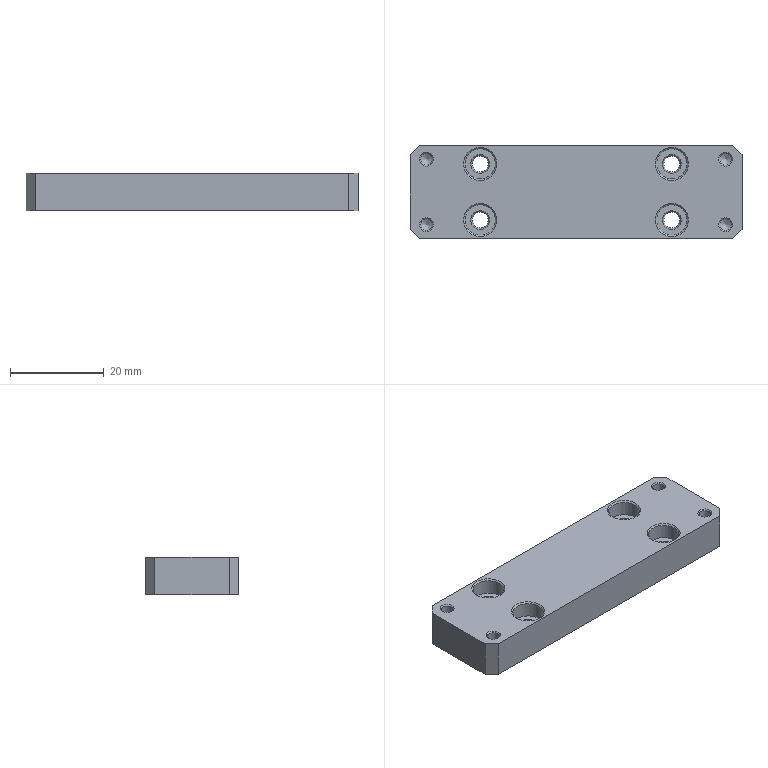Part | NX | features CBORE_HOLE 4, DATUM_CSYS 4, LINKED_CURVE 4, SIMPLE HOLE 4, SYMBOLIC_THREAD 4, SKETCH 3, HOLE PACKAGE 2, CHAMFER 1, EXTRUDE 1, LINKED_FACE 1 | 1 solid | 46 faces | box 71 x 20 x 8 mm | volume 10535 mm3 | cone 20 | plane 14 | cylinder 12 | commonest cylinder face diameters 2.5 x4 3.4 x4 6.5 x4
STEP:
#1=CARTESIAN_POINT('',(-608.186,976.556,396.282));
#2=VERTEX_POINT('',#1);
#3=CARTESIAN_POINT('',(-608.186,992.556,396.282));
#4=VERTEX_POINT('',#3);
#5=CARTESIAN_POINT('',(-608.186,974.556,396.282));
#6=DIRECTION('',(0.,1.,0.));
#7=VECTOR('',#6,1000.);
#8=LINE('',#5,#7);
#9=EDGE_CURVE('',#2,#4,#8,.T.);
#10=ORIENTED_EDGE('',*,*,#9,.T.);
#11=CARTESIAN_POINT('',(-608.186,992.556,388.282));
#12=VERTEX_POINT('',#11);
#13=CARTESIAN_POINT('',(-608.186,992.556,388.282));
#14=DIRECTION('',(0.,0.,-1.));
#15=VECTOR('',#14,1000.);
#16=LINE('',#13,#15);
#17=EDGE_CURVE('',#4,#12,#16,.T.);
#18=ORIENTED_EDGE('',*,*,#17,.T.);
#19=CARTESIAN_POINT('',(-608.186,976.556,388.282));
#20=VERTEX_POINT('',#19);
#21=CARTESIAN_POINT('',(-608.186,974.556,388.282));
#22=DIRECTION('',(0.,1.,0.));
#23=VECTOR('',#22,1000.);
#24=LINE('',#21,#23);
#25=EDGE_CURVE('',#20,#12,#24,.T.);
#26=ORIENTED_EDGE('',*,*,#25,.F.);
#27=CARTESIAN_POINT('',(-608.186,976.556,388.282));
#28=DIRECTION('',(0.,0.,1.));
#29=VECTOR('',#28,1000.);
#30=LINE('',#27,#29);
#31=EDGE_CURVE('',#20,#2,#30,.T.);
#32=ORIENTED_EDGE('',*,*,#31,.T.);
#33=EDGE_LOOP('',(#10,#18,#26,#32));
#34=FACE_BOUND('',#33,.T.);
#35=CARTESIAN_POINT('',(-608.186,974.556,388.282));
#36=DIRECTION('',(1.,0.,0.));
#37=DIRECTION('',(0.,0.,-1.));
#38=AXIS2_PLACEMENT_3D('',#35,#36,#37);
#39=PLANE('',#38);
#40=ADVANCED_FACE('',(#34),#39,.F.);
#41=CARTESIAN_POINT('',(-606.186,994.556,396.282));
#42=VERTEX_POINT('',#41);
#43=CARTESIAN_POINT('',(-539.186,994.556,396.282));
#44=VERTEX_POINT('',#43);
#45=CARTESIAN_POINT('',(-608.186,994.556,396.282));
#46=DIRECTION('',(1.,0.,0.));
#47=VECTOR('',#46,1000.);
#48=LINE('',#45,#47);
#49=EDGE_CURVE('',#42,#44,#48,.T.);
#50=ORIENTED_EDGE('',*,*,#49,.T.);
#51=CARTESIAN_POINT('',(-539.186,994.556,388.282));
#52=VERTEX_POINT('',#51);
#53=CARTESIAN_POINT('',(-539.186,994.556,388.282));
#54=DIRECTION('',(0.,0.,-1.));
#55=VECTOR('',#54,1000.);
#56=LINE('',#53,#55);
#57=EDGE_CURVE('',#44,#52,#56,.T.);
#58=ORIENTED_EDGE('',*,*,#57,.T.);
#59=CARTESIAN_POINT('',(-606.186,994.556,388.282));
#60=VERTEX_POINT('',#59);
#61=CARTESIAN_POINT('',(-608.186,994.556,388.282));
#62=DIRECTION('',(1.,0.,0.));
#63=VECTOR('',#62,1000.);
#64=LINE('',#61,#63);
#65=EDGE_CURVE('',#60,#52,#64,.T.);
#66=ORIENTED_EDGE('',*,*,#65,.F.);
#67=CARTESIAN_POINT('',(-606.186,994.556,388.282));
#68=DIRECTION('',(0.,0.,1.));
#69=VECTOR('',#68,1000.);
#70=LINE('',#67,#69);
#71=EDGE_CURVE('',#60,#42,#70,.T.);
#72=ORIENTED_EDGE('',*,*,#71,.T.);
#73=EDGE_LOOP('',(#50,#58,#66,#72));
#74=FACE_BOUND('',#73,.T.);
#75=CARTESIAN_POINT('',(-608.186,994.556,388.282));
#76=DIRECTION('',(0.,-1.,0.));
#77=DIRECTION('',(0.,0.,-1.));
#78=AXIS2_PLACEMENT_3D('',#75,#76,#77);
#79=PLANE('',#78);
#80=ADVANCED_FACE('',(#74),#79,.F.);
#81=CARTESIAN_POINT('',(-537.186,992.556,388.282));
#82=VERTEX_POINT('',#81);
#83=CARTESIAN_POINT('',(-537.186,976.556,388.282));
#84=VERTEX_POINT('',#83);
#85=CARTESIAN_POINT('',(-537.186,994.556,388.282));
#86=DIRECTION('',(0.,-1.,0.));
#87=VECTOR('',#86,1000.);
#88=LINE('',#85,#87);
#89=EDGE_CURVE('',#82,#84,#88,.T.);
#90=ORIENTED_EDGE('',*,*,#89,.F.);
#91=CARTESIAN_POINT('',(-537.186,992.556,396.282));
#92=VERTEX_POINT('',#91);
#93=CARTESIAN_POINT('',(-537.186,992.556,388.282));
#94=DIRECTION('',(0.,0.,1.));
#95=VECTOR('',#94,1000.);
#96=LINE('',#93,#95);
#97=EDGE_CURVE('',#82,#92,#96,.T.);
#98=ORIENTED_EDGE('',*,*,#97,.T.);
#99=CARTESIAN_POINT('',(-537.186,976.556,396.282));
#100=VERTEX_POINT('',#99);
#101=CARTESIAN_POINT('',(-537.186,994.556,396.282));
#102=DIRECTION('',(0.,-1.,0.));
#103=VECTOR('',#102,1000.);
#104=LINE('',#101,#103);
#105=EDGE_CURVE('',#92,#100,#104,.T.);
#106=ORIENTED_EDGE('',*,*,#105,.T.);
#107=CARTESIAN_POINT('',(-537.186,976.556,388.282));
#108=DIRECTION('',(0.,0.,-1.));
#109=VECTOR('',#108,1000.);
#110=LINE('',#107,#109);
#111=EDGE_CURVE('',#100,#84,#110,.T.);
#112=ORIENTED_EDGE('',*,*,#111,.T.);
#113=EDGE_LOOP('',(#90,#98,#106,#112));
#114=FACE_BOUND('',#113,.T.);
#115=CARTESIAN_POINT('',(-537.186,994.556,388.282));
#116=DIRECTION('',(-1.,0.,0.));
#117=DIRECTION('',(0.,0.,1.));
#118=AXIS2_PLACEMENT_3D('',#115,#116,#117);
#119=PLANE('',#118);
#120=ADVANCED_FACE('',(#114),#119,.F.);
#121=CARTESIAN_POINT('',(-539.186,974.556,388.282));
#122=VERTEX_POINT('',#121);
#123=CARTESIAN_POINT('',(-606.186,974.556,388.282));
#124=VERTEX_POINT('',#123);
#125=CARTESIAN_POINT('',(-537.186,974.556,388.282));
#126=DIRECTION('',(-1.,0.,0.));
#127=VECTOR('',#126,1000.);
#128=LINE('',#125,#127);
#129=EDGE_CURVE('',#122,#124,#128,.T.);
#130=ORIENTED_EDGE('',*,*,#129,.F.);
#131=CARTESIAN_POINT('',(-539.186,974.556,396.282));
#132=VERTEX_POINT('',#131);
#133=CARTESIAN_POINT('',(-539.186,974.556,388.282));
#134=DIRECTION('',(0.,0.,1.));
#135=VECTOR('',#134,1000.);
#136=LINE('',#133,#135);
#137=EDGE_CURVE('',#122,#132,#136,.T.);
#138=ORIENTED_EDGE('',*,*,#137,.T.);
#139=CARTESIAN_POINT('',(-606.186,974.556,396.282));
#140=VERTEX_POINT('',#139);
#141=CARTESIAN_POINT('',(-537.186,974.556,396.282));
#142=DIRECTION('',(-1.,0.,0.));
#143=VECTOR('',#142,1000.);
#144=LINE('',#141,#143);
#145=EDGE_CURVE('',#132,#140,#144,.T.);
#146=ORIENTED_EDGE('',*,*,#145,.T.);
#147=CARTESIAN_POINT('',(-606.186,974.556,388.282));
#148=DIRECTION('',(0.,0.,-1.));
#149=VECTOR('',#148,1000.);
#150=LINE('',#147,#149);
#151=EDGE_CURVE('',#140,#124,#150,.T.);
#152=ORIENTED_EDGE('',*,*,#151,.T.);
#153=EDGE_LOOP('',(#130,#138,#146,#152));
#154=FACE_BOUND('',#153,.T.);
#155=CARTESIAN_POINT('',(-537.186,974.556,388.282));
#156=DIRECTION('',(0.,1.,0.));
#157=DIRECTION('',(0.,0.,1.));
#158=AXIS2_PLACEMENT_3D('',#155,#156,#157);
#159=PLANE('',#158);
#160=ADVANCED_FACE('',(#154),#159,.F.);
#161=CARTESIAN_POINT('',(-554.186,978.556,388.282));
#162=VERTEX_POINT('',#161);
#163=CARTESIAN_POINT('',(-552.186,978.556,388.282));
#164=DIRECTION('',(0.,0.,-1.));
#165=DIRECTION('',(-1.,0.,0.));
#166=AXIS2_PLACEMENT_3D('',#163,#164,#165);
#167=CIRCLE('',#166,2.);
#168=EDGE_CURVE('',#162,#162,#167,.F.);
#169=ORIENTED_EDGE('',*,*,#168,.T.);
#170=EDGE_LOOP('',(#169));
#171=FACE_BOUND('',#170,.T.);
#172=CARTESIAN_POINT('',(-554.186,990.556,388.282));
#173=VERTEX_POINT('',#172);
#174=CARTESIAN_POINT('',(-552.186,990.556,388.282));
#175=DIRECTION('',(0.,0.,-1.));
#176=DIRECTION('',(-1.,0.,0.));
#177=AXIS2_PLACEMENT_3D('',#174,#175,#176);
#178=CIRCLE('',#177,2.);
#179=EDGE_CURVE('',#173,#173,#178,.F.);
#180=ORIENTED_EDGE('',*,*,#179,.T.);
#181=EDGE_LOOP('',(#180));
#182=FACE_BOUND('',#181,.T.);
#183=CARTESIAN_POINT('',(-595.186,978.556,388.282));
#184=VERTEX_POINT('',#183);
#185=CARTESIAN_POINT('',(-593.186,978.556,388.282));
#186=DIRECTION('',(0.,0.,-1.));
#187=DIRECTION('',(-1.,0.,0.));
#188=AXIS2_PLACEMENT_3D('',#185,#186,#187);
#189=CIRCLE('',#188,2.);
#190=EDGE_CURVE('',#184,#184,#189,.F.);
#191=ORIENTED_EDGE('',*,*,#190,.T.);
#192=EDGE_LOOP('',(#191));
#193=FACE_BOUND('',#192,.T.);
#194=CARTESIAN_POINT('',(-595.186,990.556,388.282));
#195=VERTEX_POINT('',#194);
#196=CARTESIAN_POINT('',(-593.186,990.556,388.282));
#197=DIRECTION('',(0.,0.,-1.));
#198=DIRECTION('',(-1.,0.,0.));
#199=AXIS2_PLACEMENT_3D('',#196,#197,#198);
#200=CIRCLE('',#199,2.);
#201=EDGE_CURVE('',#195,#195,#200,.F.);
#202=ORIENTED_EDGE('',*,*,#201,.T.);
#203=EDGE_LOOP('',(#202));
#204=FACE_BOUND('',#203,.T.);
#205=ORIENTED_EDGE('',*,*,#65,.T.);
#206=CARTESIAN_POINT('',(227.685,227.685,388.282));
#207=DIRECTION('',(-0.7071,0.7071,0.));
#208=VECTOR('',#207,1000.);
#209=LINE('',#206,#208);
#210=EDGE_CURVE('',#52,#82,#209,.F.);
#211=ORIENTED_EDGE('',*,*,#210,.T.);
#212=ORIENTED_EDGE('',*,*,#89,.T.);
#213=CARTESIAN_POINT('',(-756.871,756.871,388.282));
#214=DIRECTION('',(0.7071,0.7071,0.));
#215=VECTOR('',#214,1000.);
#216=LINE('',#213,#215);
#217=EDGE_CURVE('',#84,#122,#216,.F.);
#218=ORIENTED_EDGE('',*,*,#217,.T.);
#219=ORIENTED_EDGE('',*,*,#129,.T.);
#220=CARTESIAN_POINT('',(184.185,184.185,388.282));
#221=DIRECTION('',(0.7071,-0.7071,0.));
#222=VECTOR('',#221,1000.);
#223=LINE('',#220,#222);
#224=EDGE_CURVE('',#124,#20,#223,.F.);
#225=ORIENTED_EDGE('',*,*,#224,.T.);
#226=ORIENTED_EDGE('',*,*,#25,.T.);
#227=CARTESIAN_POINT('',(-800.371,800.371,388.282));
#228=DIRECTION('',(-0.7071,-0.7071,0.));
#229=VECTOR('',#228,1000.);
#230=LINE('',#227,#229);
#231=EDGE_CURVE('',#12,#60,#230,.F.);
#232=ORIENTED_EDGE('',*,*,#231,.T.);
#233=EDGE_LOOP('',(#205,#211,#212,#218,#219,#225,#226,#232));
#234=FACE_BOUND('',#233,.T.);
#235=CARTESIAN_POINT('',(0.,0.,388.282));
#236=DIRECTION('',(0.,0.,-1.));
#237=DIRECTION('',(-1.,0.,0.));
#238=AXIS2_PLACEMENT_3D('',#235,#236,#237);
#239=PLANE('',#238);
#240=ADVANCED_FACE('',(#171,#182,#193,#204,#234),#239,.T.);
#241=CARTESIAN_POINT('',(-555.736,978.556,396.282));
#242=VERTEX_POINT('',#241);
#243=CARTESIAN_POINT('',(-552.186,978.556,396.282));
#244=DIRECTION('',(0.,0.,-1.));
#245=DIRECTION('',(-1.,0.,0.));
#246=AXIS2_PLACEMENT_3D('',#243,#244,#245);
#247=CIRCLE('',#246,3.55);
#248=EDGE_CURVE('',#242,#242,#247,.T.);
#249=ORIENTED_EDGE('',*,*,#248,.T.);
#250=EDGE_LOOP('',(#249));
#251=FACE_BOUND('',#250,.T.);
#252=CARTESIAN_POINT('',(-555.736,990.556,396.282));
#253=VERTEX_POINT('',#252);
#254=CARTESIAN_POINT('',(-552.186,990.556,396.282));
#255=DIRECTION('',(0.,0.,-1.));
#256=DIRECTION('',(-1.,0.,0.));
#257=AXIS2_PLACEMENT_3D('',#254,#255,#256);
#258=CIRCLE('',#257,3.55);
#259=EDGE_CURVE('',#253,#253,#258,.T.);
#260=ORIENTED_EDGE('',*,*,#259,.T.);
#261=EDGE_LOOP('',(#260));
#262=FACE_BOUND('',#261,.T.);
#263=CARTESIAN_POINT('',(-596.736,978.556,396.282));
#264=VERTEX_POINT('',#263);
#265=CARTESIAN_POINT('',(-593.186,978.556,396.282));
#266=DIRECTION('',(0.,0.,-1.));
#267=DIRECTION('',(-1.,0.,0.));
#268=AXIS2_PLACEMENT_3D('',#265,#266,#267);
#269=CIRCLE('',#268,3.55);
#270=EDGE_CURVE('',#264,#264,#269,.T.);
#271=ORIENTED_EDGE('',*,*,#270,.T.);
#272=EDGE_LOOP('',(#271));
#273=FACE_BOUND('',#272,.T.);
#274=CARTESIAN_POINT('',(-596.736,990.556,396.282));
#275=VERTEX_POINT('',#274);
#276=CARTESIAN_POINT('',(-593.186,990.556,396.282));
#277=DIRECTION('',(0.,0.,-1.));
#278=DIRECTION('',(-1.,0.,0.));
#279=AXIS2_PLACEMENT_3D('',#276,#277,#278);
#280=CIRCLE('',#279,3.55);
#281=EDGE_CURVE('',#275,#275,#280,.T.);
#282=ORIENTED_EDGE('',*,*,#281,.T.);
#283=EDGE_LOOP('',(#282));
#284=FACE_BOUND('',#283,.T.);
#285=CARTESIAN_POINT('',(-542.186,977.556,396.282));
#286=VERTEX_POINT('',#285);
#287=CARTESIAN_POINT('',(-540.686,977.556,396.282));
#288=DIRECTION('',(0.,0.,-1.));
#289=DIRECTION('',(-1.,0.,0.));
#290=AXIS2_PLACEMENT_3D('',#287,#288,#289);
#291=CIRCLE('',#290,1.5);
#292=EDGE_CURVE('',#286,#286,#291,.T.);
#293=ORIENTED_EDGE('',*,*,#292,.T.);
#294=EDGE_LOOP('',(#293));
#295=FACE_BOUND('',#294,.T.);
#296=CARTESIAN_POINT('',(-542.186,991.556,396.282));
#297=VERTEX_POINT('',#296);
#298=CARTESIAN_POINT('',(-540.686,991.556,396.282));
#299=DIRECTION('',(0.,0.,-1.));
#300=DIRECTION('',(-1.,0.,0.));
#301=AXIS2_PLACEMENT_3D('',#298,#299,#300);
#302=CIRCLE('',#301,1.5);
#303=EDGE_CURVE('',#297,#297,#302,.T.);
#304=ORIENTED_EDGE('',*,*,#303,.T.);
#305=EDGE_LOOP('',(#304));
#306=FACE_BOUND('',#305,.T.);
#307=CARTESIAN_POINT('',(-606.186,977.561,396.282));
#308=VERTEX_POINT('',#307);
#309=CARTESIAN_POINT('',(-604.686,977.561,396.282));
#310=DIRECTION('',(0.,0.,-1.));
#311=DIRECTION('',(-1.,0.,0.));
#312=AXIS2_PLACEMENT_3D('',#309,#310,#311);
#313=CIRCLE('',#312,1.5);
#314=EDGE_CURVE('',#308,#308,#313,.T.);
#315=ORIENTED_EDGE('',*,*,#314,.T.);
#316=EDGE_LOOP('',(#315));
#317=FACE_BOUND('',#316,.T.);
#318=CARTESIAN_POINT('',(-606.186,991.561,396.282));
#319=VERTEX_POINT('',#318);
#320=CARTESIAN_POINT('',(-604.686,991.561,396.282));
#321=DIRECTION('',(0.,0.,-1.));
#322=DIRECTION('',(-1.,0.,0.));
#323=AXIS2_PLACEMENT_3D('',#320,#321,#322);
#324=CIRCLE('',#323,1.5);
#325=EDGE_CURVE('',#319,#319,#324,.T.);
#326=ORIENTED_EDGE('',*,*,#325,.T.);
#327=EDGE_LOOP('',(#326));
#328=FACE_BOUND('',#327,.T.);
#329=ORIENTED_EDGE('',*,*,#105,.F.);
#330=CARTESIAN_POINT('',(-537.186,992.556,396.282));
#331=DIRECTION('',(0.7071,-0.7071,0.));
#332=VECTOR('',#331,1000.);
#333=LINE('',#330,#332);
#334=EDGE_CURVE('',#92,#44,#333,.F.);
#335=ORIENTED_EDGE('',*,*,#334,.T.);
#336=ORIENTED_EDGE('',*,*,#49,.F.);
#337=CARTESIAN_POINT('',(-606.186,994.556,396.282));
#338=DIRECTION('',(0.7071,0.7071,0.));
#339=VECTOR('',#338,1000.);
#340=LINE('',#337,#339);
#341=EDGE_CURVE('',#42,#4,#340,.F.);
#342=ORIENTED_EDGE('',*,*,#341,.T.);
#343=ORIENTED_EDGE('',*,*,#9,.F.);
#344=CARTESIAN_POINT('',(-608.186,976.556,396.282));
#345=DIRECTION('',(-0.7071,0.7071,0.));
#346=VECTOR('',#345,1000.);
#347=LINE('',#344,#346);
#348=EDGE_CURVE('',#2,#140,#347,.F.);
#349=ORIENTED_EDGE('',*,*,#348,.T.);
#350=ORIENTED_EDGE('',*,*,#145,.F.);
#351=CARTESIAN_POINT('',(-539.186,974.556,396.282));
#352=DIRECTION('',(-0.7071,-0.7071,0.));
#353=VECTOR('',#352,1000.);
#354=LINE('',#351,#353);
#355=EDGE_CURVE('',#132,#100,#354,.F.);
#356=ORIENTED_EDGE('',*,*,#355,.T.);
#357=EDGE_LOOP('',(#329,#335,#336,#342,#343,#349,#350,#356));
#358=FACE_BOUND('',#357,.T.);
#359=CARTESIAN_POINT('',(0.,0.,396.282));
#360=DIRECTION('',(0.,0.,-1.));
#361=DIRECTION('',(-1.,0.,0.));
#362=AXIS2_PLACEMENT_3D('',#359,#360,#361);
#363=PLANE('',#362);
#364=ADVANCED_FACE('',(#251,#262,#273,#284,#295,#306,#317,#328,#358),#363,.F.);
#365=CARTESIAN_POINT('',(-605.936,991.561,390.282));
#366=VERTEX_POINT('',#365);
#367=CARTESIAN_POINT('',(-604.686,991.561,390.282));
#368=DIRECTION('',(0.,0.,-1.));
#369=DIRECTION('',(-1.,0.,0.));
#370=AXIS2_PLACEMENT_3D('',#367,#368,#369);
#371=CIRCLE('',#370,1.25);
#372=EDGE_CURVE('',#366,#366,#371,.F.);
#373=ORIENTED_EDGE('',*,*,#372,.T.);
#374=EDGE_LOOP('',(#373));
#375=FACE_BOUND('',#374,.T.);
#376=CARTESIAN_POINT('',(-604.686,991.561,389.531));
#377=VERTEX_POINT('',#376);
#378=VERTEX_LOOP('',#377);
#379=FACE_BOUND('',#378,.T.);
#380=CARTESIAN_POINT('',(-604.686,991.561,390.282));
#381=DIRECTION('',(0.,0.,1.));
#382=DIRECTION('',(1.,0.,0.));
#383=AXIS2_PLACEMENT_3D('',#380,#381,#382);
#384=CONICAL_SURFACE('',#383,1.25,1.03);
#385=ADVANCED_FACE('',(#375,#379),#384,.F.);
#386=CARTESIAN_POINT('',(-605.936,991.561,396.032));
#387=VERTEX_POINT('',#386);
#388=CARTESIAN_POINT('',(-604.686,991.561,396.032));
#389=DIRECTION('',(0.,0.,-1.));
#390=DIRECTION('',(-1.,0.,0.));
#391=AXIS2_PLACEMENT_3D('',#388,#389,#390);
#392=CIRCLE('',#391,1.25);
#393=EDGE_CURVE('',#387,#387,#392,.F.);
#394=ORIENTED_EDGE('',*,*,#393,.T.);
#395=EDGE_LOOP('',(#394));
#396=FACE_BOUND('',#395,.T.);
#397=ORIENTED_EDGE('',*,*,#372,.F.);
#398=EDGE_LOOP('',(#397));
#399=FACE_BOUND('',#398,.T.);
#400=CARTESIAN_POINT('',(-604.686,991.561,396.282));
#401=DIRECTION('',(0.,0.,-1.));
#402=DIRECTION('',(-1.,0.,0.));
#403=AXIS2_PLACEMENT_3D('',#400,#401,#402);
#404=CYLINDRICAL_SURFACE('',#403,1.25);
#405=ADVANCED_FACE('',(#396,#399),#404,.F.);
#406=ORIENTED_EDGE('',*,*,#393,.F.);
#407=EDGE_LOOP('',(#406));
#408=FACE_BOUND('',#407,.T.);
#409=ORIENTED_EDGE('',*,*,#325,.F.);
#410=EDGE_LOOP('',(#409));
#411=FACE_BOUND('',#410,.T.);
#412=CARTESIAN_POINT('',(-604.686,991.561,396.282));
#413=DIRECTION('',(0.,0.,1.));
#414=DIRECTION('',(1.,0.,0.));
#415=AXIS2_PLACEMENT_3D('',#412,#413,#414);
#416=CONICAL_SURFACE('',#415,1.5,0.7854);
#417=ADVANCED_FACE('',(#408,#411),#416,.F.);
#418=CARTESIAN_POINT('',(-605.936,977.561,390.282));
#419=VERTEX_POINT('',#418);
#420=CARTESIAN_POINT('',(-604.686,977.561,390.282));
#421=DIRECTION('',(0.,0.,-1.));
#422=DIRECTION('',(-1.,0.,0.));
#423=AXIS2_PLACEMENT_3D('',#420,#421,#422);
#424=CIRCLE('',#423,1.25);
#425=EDGE_CURVE('',#419,#419,#424,.F.);
#426=ORIENTED_EDGE('',*,*,#425,.T.);
#427=EDGE_LOOP('',(#426));
#428=FACE_BOUND('',#427,.T.);
#429=CARTESIAN_POINT('',(-604.686,977.561,389.531));
#430=VERTEX_POINT('',#429);
#431=VERTEX_LOOP('',#430);
#432=FACE_BOUND('',#431,.T.);
#433=CARTESIAN_POINT('',(-604.686,977.561,390.282));
#434=DIRECTION('',(0.,0.,1.));
#435=DIRECTION('',(1.,0.,0.));
#436=AXIS2_PLACEMENT_3D('',#433,#434,#435);
#437=CONICAL_SURFACE('',#436,1.25,1.03);
#438=ADVANCED_FACE('',(#428,#432),#437,.F.);
#439=CARTESIAN_POINT('',(-605.936,977.561,396.032));
#440=VERTEX_POINT('',#439);
#441=CARTESIAN_POINT('',(-604.686,977.561,396.032));
#442=DIRECTION('',(0.,0.,-1.));
#443=DIRECTION('',(-1.,0.,0.));
#444=AXIS2_PLACEMENT_3D('',#441,#442,#443);
#445=CIRCLE('',#444,1.25);
#446=EDGE_CURVE('',#440,#440,#445,.F.);
#447=ORIENTED_EDGE('',*,*,#446,.T.);
#448=EDGE_LOOP('',(#447));
#449=FACE_BOUND('',#448,.T.);
#450=ORIENTED_EDGE('',*,*,#425,.F.);
#451=EDGE_LOOP('',(#450));
#452=FACE_BOUND('',#451,.T.);
#453=CARTESIAN_POINT('',(-604.686,977.561,396.282));
#454=DIRECTION('',(0.,0.,-1.));
#455=DIRECTION('',(-1.,0.,0.));
#456=AXIS2_PLACEMENT_3D('',#453,#454,#455);
#457=CYLINDRICAL_SURFACE('',#456,1.25);
#458=ADVANCED_FACE('',(#449,#452),#457,.F.);
#459=ORIENTED_EDGE('',*,*,#446,.F.);
#460=EDGE_LOOP('',(#459));
#461=FACE_BOUND('',#460,.T.);
#462=ORIENTED_EDGE('',*,*,#314,.F.);
#463=EDGE_LOOP('',(#462));
#464=FACE_BOUND('',#463,.T.);
#465=CARTESIAN_POINT('',(-604.686,977.561,396.282));
#466=DIRECTION('',(0.,0.,1.));
#467=DIRECTION('',(1.,0.,0.));
#468=AXIS2_PLACEMENT_3D('',#465,#466,#467);
#469=CONICAL_SURFACE('',#468,1.5,0.7854);
#470=ADVANCED_FACE('',(#461,#464),#469,.F.);
#471=CARTESIAN_POINT('',(-541.936,991.556,390.282));
#472=VERTEX_POINT('',#471);
#473=CARTESIAN_POINT('',(-540.686,991.556,390.282));
#474=DIRECTION('',(0.,0.,-1.));
#475=DIRECTION('',(-1.,0.,0.));
#476=AXIS2_PLACEMENT_3D('',#473,#474,#475);
#477=CIRCLE('',#476,1.25);
#478=EDGE_CURVE('',#472,#472,#477,.F.);
#479=ORIENTED_EDGE('',*,*,#478,.T.);
#480=EDGE_LOOP('',(#479));
#481=FACE_BOUND('',#480,.T.);
#482=CARTESIAN_POINT('',(-540.686,991.556,389.531));
#483=VERTEX_POINT('',#482);
#484=VERTEX_LOOP('',#483);
#485=FACE_BOUND('',#484,.T.);
#486=CARTESIAN_POINT('',(-540.686,991.556,390.282));
#487=DIRECTION('',(0.,0.,1.));
#488=DIRECTION('',(1.,0.,0.));
#489=AXIS2_PLACEMENT_3D('',#486,#487,#488);
#490=CONICAL_SURFACE('',#489,1.25,1.03);
#491=ADVANCED_FACE('',(#481,#485),#490,.F.);
#492=CARTESIAN_POINT('',(-541.936,991.556,396.032));
#493=VERTEX_POINT('',#492);
#494=CARTESIAN_POINT('',(-540.686,991.556,396.032));
#495=DIRECTION('',(0.,0.,-1.));
#496=DIRECTION('',(-1.,0.,0.));
#497=AXIS2_PLACEMENT_3D('',#494,#495,#496);
#498=CIRCLE('',#497,1.25);
#499=EDGE_CURVE('',#493,#493,#498,.F.);
#500=ORIENTED_EDGE('',*,*,#499,.T.);
#501=EDGE_LOOP('',(#500));
#502=FACE_BOUND('',#501,.T.);
#503=ORIENTED_EDGE('',*,*,#478,.F.);
#504=EDGE_LOOP('',(#503));
#505=FACE_BOUND('',#504,.T.);
#506=CARTESIAN_POINT('',(-540.686,991.556,396.282));
#507=DIRECTION('',(0.,0.,-1.));
#508=DIRECTION('',(-1.,0.,0.));
#509=AXIS2_PLACEMENT_3D('',#506,#507,#508);
#510=CYLINDRICAL_SURFACE('',#509,1.25);
#511=ADVANCED_FACE('',(#502,#505),#510,.F.);
#512=ORIENTED_EDGE('',*,*,#499,.F.);
#513=EDGE_LOOP('',(#512));
#514=FACE_BOUND('',#513,.T.);
#515=ORIENTED_EDGE('',*,*,#303,.F.);
#516=EDGE_LOOP('',(#515));
#517=FACE_BOUND('',#516,.T.);
#518=CARTESIAN_POINT('',(-540.686,991.556,396.282));
#519=DIRECTION('',(0.,0.,1.));
#520=DIRECTION('',(1.,0.,0.));
#521=AXIS2_PLACEMENT_3D('',#518,#519,#520);
#522=CONICAL_SURFACE('',#521,1.5,0.7854);
#523=ADVANCED_FACE('',(#514,#517),#522,.F.);
#524=CARTESIAN_POINT('',(-541.936,977.556,390.282));
#525=VERTEX_POINT('',#524);
#526=CARTESIAN_POINT('',(-540.686,977.556,390.282));
#527=DIRECTION('',(0.,0.,-1.));
#528=DIRECTION('',(-1.,0.,0.));
#529=AXIS2_PLACEMENT_3D('',#526,#527,#528);
#530=CIRCLE('',#529,1.25);
#531=EDGE_CURVE('',#525,#525,#530,.F.);
#532=ORIENTED_EDGE('',*,*,#531,.T.);
#533=EDGE_LOOP('',(#532));
#534=FACE_BOUND('',#533,.T.);
#535=CARTESIAN_POINT('',(-540.686,977.556,389.531));
#536=VERTEX_POINT('',#535);
#537=VERTEX_LOOP('',#536);
#538=FACE_BOUND('',#537,.T.);
#539=CARTESIAN_POINT('',(-540.686,977.556,390.282));
#540=DIRECTION('',(0.,0.,1.));
#541=DIRECTION('',(1.,0.,0.));
#542=AXIS2_PLACEMENT_3D('',#539,#540,#541);
#543=CONICAL_SURFACE('',#542,1.25,1.03);
#544=ADVANCED_FACE('',(#534,#538),#543,.F.);
#545=CARTESIAN_POINT('',(-541.936,977.556,396.032));
#546=VERTEX_POINT('',#545);
#547=CARTESIAN_POINT('',(-540.686,977.556,396.032));
#548=DIRECTION('',(0.,0.,-1.));
#549=DIRECTION('',(-1.,0.,0.));
#550=AXIS2_PLACEMENT_3D('',#547,#548,#549);
#551=CIRCLE('',#550,1.25);
#552=EDGE_CURVE('',#546,#546,#551,.F.);
#553=ORIENTED_EDGE('',*,*,#552,.T.);
#554=EDGE_LOOP('',(#553));
#555=FACE_BOUND('',#554,.T.);
#556=ORIENTED_EDGE('',*,*,#531,.F.);
#557=EDGE_LOOP('',(#556));
#558=FACE_BOUND('',#557,.T.);
#559=CARTESIAN_POINT('',(-540.686,977.556,396.282));
#560=DIRECTION('',(0.,0.,-1.));
#561=DIRECTION('',(-1.,0.,0.));
#562=AXIS2_PLACEMENT_3D('',#559,#560,#561);
#563=CYLINDRICAL_SURFACE('',#562,1.25);
#564=ADVANCED_FACE('',(#555,#558),#563,.F.);
#565=ORIENTED_EDGE('',*,*,#552,.F.);
#566=EDGE_LOOP('',(#565));
#567=FACE_BOUND('',#566,.T.);
#568=ORIENTED_EDGE('',*,*,#292,.F.);
#569=EDGE_LOOP('',(#568));
#570=FACE_BOUND('',#569,.T.);
#571=CARTESIAN_POINT('',(-540.686,977.556,396.282));
#572=DIRECTION('',(0.,0.,1.));
#573=DIRECTION('',(1.,0.,0.));
#574=AXIS2_PLACEMENT_3D('',#571,#572,#573);
#575=CONICAL_SURFACE('',#574,1.5,0.7854);
#576=ADVANCED_FACE('',(#567,#570),#575,.F.);
#577=ORIENTED_EDGE('',*,*,#210,.F.);
#578=ORIENTED_EDGE('',*,*,#57,.F.);
#579=ORIENTED_EDGE('',*,*,#334,.F.);
#580=ORIENTED_EDGE('',*,*,#97,.F.);
#581=EDGE_LOOP('',(#577,#578,#579,#580));
#582=FACE_BOUND('',#581,.T.);
#583=CARTESIAN_POINT('',(-537.186,992.556,388.282));
#584=DIRECTION('',(-0.7071,-0.7071,0.));
#585=DIRECTION('',(0.,0.,1.));
#586=AXIS2_PLACEMENT_3D('',#583,#584,#585);
#587=PLANE('',#586);
#588=ADVANCED_FACE('',(#582),#587,.F.);
#589=ORIENTED_EDGE('',*,*,#217,.F.);
#590=ORIENTED_EDGE('',*,*,#111,.F.);
#591=ORIENTED_EDGE('',*,*,#355,.F.);
#592=ORIENTED_EDGE('',*,*,#137,.F.);
#593=EDGE_LOOP('',(#589,#590,#591,#592));
#594=FACE_BOUND('',#593,.T.);
#595=CARTESIAN_POINT('',(-539.186,974.556,388.282));
#596=DIRECTION('',(-0.7071,0.7071,0.));
#597=DIRECTION('',(0.,0.,1.));
#598=AXIS2_PLACEMENT_3D('',#595,#596,#597);
#599=PLANE('',#598);
#600=ADVANCED_FACE('',(#594),#599,.F.);
#601=ORIENTED_EDGE('',*,*,#231,.F.);
#602=ORIENTED_EDGE('',*,*,#17,.F.);
#603=ORIENTED_EDGE('',*,*,#341,.F.);
#604=ORIENTED_EDGE('',*,*,#71,.F.);
#605=EDGE_LOOP('',(#601,#602,#603,#604));
#606=FACE_BOUND('',#605,.T.);
#607=CARTESIAN_POINT('',(-606.186,994.556,388.282));
#608=DIRECTION('',(0.7071,-0.7071,0.));
#609=DIRECTION('',(0.,0.,1.));
#610=AXIS2_PLACEMENT_3D('',#607,#608,#609);
#611=PLANE('',#610);
#612=ADVANCED_FACE('',(#606),#611,.F.);
#613=ORIENTED_EDGE('',*,*,#224,.F.);
#614=ORIENTED_EDGE('',*,*,#151,.F.);
#615=ORIENTED_EDGE('',*,*,#348,.F.);
#616=ORIENTED_EDGE('',*,*,#31,.F.);
#617=EDGE_LOOP('',(#613,#614,#615,#616));
#618=FACE_BOUND('',#617,.T.);
#619=CARTESIAN_POINT('',(-608.186,976.556,388.282));
#620=DIRECTION('',(0.7071,0.7071,0.));
#621=DIRECTION('',(0.,0.,1.));
#622=AXIS2_PLACEMENT_3D('',#619,#620,#621);
#623=PLANE('',#622);
#624=ADVANCED_FACE('',(#618),#623,.F.);
#625=CARTESIAN_POINT('',(-594.886,990.556,388.582));
#626=VERTEX_POINT('',#625);
#627=CARTESIAN_POINT('',(-593.186,990.556,388.582));
#628=DIRECTION('',(0.,0.,-1.));
#629=DIRECTION('',(-1.,0.,0.));
#630=AXIS2_PLACEMENT_3D('',#627,#628,#629);
#631=CIRCLE('',#630,1.7);
#632=EDGE_CURVE('',#626,#626,#631,.T.);
#633=ORIENTED_EDGE('',*,*,#632,.T.);
#634=EDGE_LOOP('',(#633));
#635=FACE_BOUND('',#634,.T.);
#636=CARTESIAN_POINT('',(-594.886,990.556,392.262));
#637=VERTEX_POINT('',#636);
#638=CARTESIAN_POINT('',(-593.186,990.556,392.262));
#639=DIRECTION('',(0.,0.,-1.));
#640=DIRECTION('',(-1.,0.,0.));
#641=AXIS2_PLACEMENT_3D('',#638,#639,#640);
#642=CIRCLE('',#641,1.7);
#643=EDGE_CURVE('',#637,#637,#642,.F.);
#644=ORIENTED_EDGE('',*,*,#643,.T.);
#645=EDGE_LOOP('',(#644));
#646=FACE_BOUND('',#645,.T.);
#647=CARTESIAN_POINT('',(-593.186,990.556,346.282));
#648=DIRECTION('',(0.,0.,-1.));
#649=DIRECTION('',(-1.,0.,0.));
#650=AXIS2_PLACEMENT_3D('',#647,#648,#649);
#651=CYLINDRICAL_SURFACE('',#650,1.7);
#652=ADVANCED_FACE('',(#635,#646),#651,.F.);
#653=CARTESIAN_POINT('',(-595.186,990.556,392.782));
#654=VERTEX_POINT('',#653);
#655=CARTESIAN_POINT('',(-593.186,990.556,392.782));
#656=DIRECTION('',(0.,0.,-1.));
#657=DIRECTION('',(-1.,0.,0.));
#658=AXIS2_PLACEMENT_3D('',#655,#656,#657);
#659=CIRCLE('',#658,2.);
#660=EDGE_CURVE('',#654,#654,#659,.T.);
#661=ORIENTED_EDGE('',*,*,#660,.T.);
#662=EDGE_LOOP('',(#661));
#663=FACE_BOUND('',#662,.T.);
#664=CARTESIAN_POINT('',(-596.436,990.556,392.782));
#665=VERTEX_POINT('',#664);
#666=CARTESIAN_POINT('',(-593.186,990.556,392.782));
#667=DIRECTION('',(0.,0.,-1.));
#668=DIRECTION('',(-1.,0.,0.));
#669=AXIS2_PLACEMENT_3D('',#666,#667,#668);
#670=CIRCLE('',#669,3.25);
#671=EDGE_CURVE('',#665,#665,#670,.F.);
#672=ORIENTED_EDGE('',*,*,#671,.T.);
#673=EDGE_LOOP('',(#672));
#674=FACE_BOUND('',#673,.T.);
#675=CARTESIAN_POINT('',(-593.186,990.556,392.782));
#676=DIRECTION('',(0.,0.,-1.));
#677=DIRECTION('',(-1.,0.,0.));
#678=AXIS2_PLACEMENT_3D('',#675,#676,#677);
#679=PLANE('',#678);
#680=ADVANCED_FACE('',(#663,#674),#679,.F.);
#681=CARTESIAN_POINT('',(-596.436,990.556,395.982));
#682=VERTEX_POINT('',#681);
#683=CARTESIAN_POINT('',(-593.186,990.556,395.982));
#684=DIRECTION('',(0.,0.,-1.));
#685=DIRECTION('',(-1.,0.,0.));
#686=AXIS2_PLACEMENT_3D('',#683,#684,#685);
#687=CIRCLE('',#686,3.25);
#688=EDGE_CURVE('',#682,#682,#687,.F.);
#689=ORIENTED_EDGE('',*,*,#688,.T.);
#690=EDGE_LOOP('',(#689));
#691=FACE_BOUND('',#690,.T.);
#692=ORIENTED_EDGE('',*,*,#671,.F.);
#693=EDGE_LOOP('',(#692));
#694=FACE_BOUND('',#693,.T.);
#695=CARTESIAN_POINT('',(-593.186,990.556,396.282));
#696=DIRECTION('',(0.,0.,-1.));
#697=DIRECTION('',(-1.,0.,0.));
#698=AXIS2_PLACEMENT_3D('',#695,#696,#697);
#699=CYLINDRICAL_SURFACE('',#698,3.25);
#700=ADVANCED_FACE('',(#691,#694),#699,.F.);
#701=ORIENTED_EDGE('',*,*,#660,.F.);
#702=EDGE_LOOP('',(#701));
#703=FACE_BOUND('',#702,.T.);
#704=ORIENTED_EDGE('',*,*,#643,.F.);
#705=EDGE_LOOP('',(#704));
#706=FACE_BOUND('',#705,.T.);
#707=CARTESIAN_POINT('',(-593.186,990.556,392.262));
#708=DIRECTION('',(0.,0.,1.));
#709=DIRECTION('',(1.,0.,0.));
#710=AXIS2_PLACEMENT_3D('',#707,#708,#709);
#711=CONICAL_SURFACE('',#710,1.7,0.5236);
#712=ADVANCED_FACE('',(#703,#706),#711,.F.);
#713=ORIENTED_EDGE('',*,*,#688,.F.);
#714=EDGE_LOOP('',(#713));
#715=FACE_BOUND('',#714,.T.);
#716=ORIENTED_EDGE('',*,*,#281,.F.);
#717=EDGE_LOOP('',(#716));
#718=FACE_BOUND('',#717,.T.);
#719=CARTESIAN_POINT('',(-593.186,990.556,396.282));
#720=DIRECTION('',(0.,0.,1.));
#721=DIRECTION('',(1.,0.,0.));
#722=AXIS2_PLACEMENT_3D('',#719,#720,#721);
#723=CONICAL_SURFACE('',#722,3.55,0.7854);
#724=ADVANCED_FACE('',(#715,#718),#723,.F.);
#725=ORIENTED_EDGE('',*,*,#201,.F.);
#726=EDGE_LOOP('',(#725));
#727=FACE_BOUND('',#726,.T.);
#728=ORIENTED_EDGE('',*,*,#632,.F.);
#729=EDGE_LOOP('',(#728));
#730=FACE_BOUND('',#729,.T.);
#731=CARTESIAN_POINT('',(-593.186,990.556,388.582));
#732=DIRECTION('',(0.,0.,-1.));
#733=DIRECTION('',(-1.,0.,0.));
#734=AXIS2_PLACEMENT_3D('',#731,#732,#733);
#735=CONICAL_SURFACE('',#734,1.7,0.7854);
#736=ADVANCED_FACE('',(#727,#730),#735,.F.);
#737=CARTESIAN_POINT('',(-594.886,978.556,388.582));
#738=VERTEX_POINT('',#737);
#739=CARTESIAN_POINT('',(-593.186,978.556,388.582));
#740=DIRECTION('',(0.,0.,-1.));
#741=DIRECTION('',(-1.,0.,0.));
#742=AXIS2_PLACEMENT_3D('',#739,#740,#741);
#743=CIRCLE('',#742,1.7);
#744=EDGE_CURVE('',#738,#738,#743,.T.);
#745=ORIENTED_EDGE('',*,*,#744,.T.);
#746=EDGE_LOOP('',(#745));
#747=FACE_BOUND('',#746,.T.);
#748=CARTESIAN_POINT('',(-594.886,978.556,392.262));
#749=VERTEX_POINT('',#748);
#750=CARTESIAN_POINT('',(-593.186,978.556,392.262));
#751=DIRECTION('',(0.,0.,-1.));
#752=DIRECTION('',(-1.,0.,0.));
#753=AXIS2_PLACEMENT_3D('',#750,#751,#752);
#754=CIRCLE('',#753,1.7);
#755=EDGE_CURVE('',#749,#749,#754,.F.);
#756=ORIENTED_EDGE('',*,*,#755,.T.);
#757=EDGE_LOOP('',(#756));
#758=FACE_BOUND('',#757,.T.);
#759=CARTESIAN_POINT('',(-593.186,978.556,346.282));
#760=DIRECTION('',(0.,0.,-1.));
#761=DIRECTION('',(-1.,0.,0.));
#762=AXIS2_PLACEMENT_3D('',#759,#760,#761);
#763=CYLINDRICAL_SURFACE('',#762,1.7);
#764=ADVANCED_FACE('',(#747,#758),#763,.F.);
#765=CARTESIAN_POINT('',(-595.186,978.556,392.782));
#766=VERTEX_POINT('',#765);
#767=CARTESIAN_POINT('',(-593.186,978.556,392.782));
#768=DIRECTION('',(0.,0.,-1.));
#769=DIRECTION('',(-1.,0.,0.));
#770=AXIS2_PLACEMENT_3D('',#767,#768,#769);
#771=CIRCLE('',#770,2.);
#772=EDGE_CURVE('',#766,#766,#771,.T.);
#773=ORIENTED_EDGE('',*,*,#772,.T.);
#774=EDGE_LOOP('',(#773));
#775=FACE_BOUND('',#774,.T.);
#776=CARTESIAN_POINT('',(-596.436,978.556,392.782));
#777=VERTEX_POINT('',#776);
#778=CARTESIAN_POINT('',(-593.186,978.556,392.782));
#779=DIRECTION('',(0.,0.,-1.));
#780=DIRECTION('',(-1.,0.,0.));
#781=AXIS2_PLACEMENT_3D('',#778,#779,#780);
#782=CIRCLE('',#781,3.25);
#783=EDGE_CURVE('',#777,#777,#782,.F.);
#784=ORIENTED_EDGE('',*,*,#783,.T.);
#785=EDGE_LOOP('',(#784));
#786=FACE_BOUND('',#785,.T.);
#787=CARTESIAN_POINT('',(-593.186,978.556,392.782));
#788=DIRECTION('',(0.,0.,-1.));
#789=DIRECTION('',(-1.,0.,0.));
#790=AXIS2_PLACEMENT_3D('',#787,#788,#789);
#791=PLANE('',#790);
#792=ADVANCED_FACE('',(#775,#786),#791,.F.);
#793=CARTESIAN_POINT('',(-596.436,978.556,395.982));
#794=VERTEX_POINT('',#793);
#795=CARTESIAN_POINT('',(-593.186,978.556,395.982));
#796=DIRECTION('',(0.,0.,-1.));
#797=DIRECTION('',(-1.,0.,0.));
#798=AXIS2_PLACEMENT_3D('',#795,#796,#797);
#799=CIRCLE('',#798,3.25);
#800=EDGE_CURVE('',#794,#794,#799,.F.);
#801=ORIENTED_EDGE('',*,*,#800,.T.);
#802=EDGE_LOOP('',(#801));
#803=FACE_BOUND('',#802,.T.);
#804=ORIENTED_EDGE('',*,*,#783,.F.);
#805=EDGE_LOOP('',(#804));
#806=FACE_BOUND('',#805,.T.);
#807=CARTESIAN_POINT('',(-593.186,978.556,396.282));
#808=DIRECTION('',(0.,0.,-1.));
#809=DIRECTION('',(-1.,0.,0.));
#810=AXIS2_PLACEMENT_3D('',#807,#808,#809);
#811=CYLINDRICAL_SURFACE('',#810,3.25);
#812=ADVANCED_FACE('',(#803,#806),#811,.F.);
#813=ORIENTED_EDGE('',*,*,#772,.F.);
#814=EDGE_LOOP('',(#813));
#815=FACE_BOUND('',#814,.T.);
#816=ORIENTED_EDGE('',*,*,#755,.F.);
#817=EDGE_LOOP('',(#816));
#818=FACE_BOUND('',#817,.T.);
#819=CARTESIAN_POINT('',(-593.186,978.556,392.262));
#820=DIRECTION('',(0.,0.,1.));
#821=DIRECTION('',(1.,0.,0.));
#822=AXIS2_PLACEMENT_3D('',#819,#820,#821);
#823=CONICAL_SURFACE('',#822,1.7,0.5236);
#824=ADVANCED_FACE('',(#815,#818),#823,.F.);
#825=ORIENTED_EDGE('',*,*,#800,.F.);
#826=EDGE_LOOP('',(#825));
#827=FACE_BOUND('',#826,.T.);
#828=ORIENTED_EDGE('',*,*,#270,.F.);
#829=EDGE_LOOP('',(#828));
#830=FACE_BOUND('',#829,.T.);
#831=CARTESIAN_POINT('',(-593.186,978.556,396.282));
#832=DIRECTION('',(0.,0.,1.));
#833=DIRECTION('',(1.,0.,0.));
#834=AXIS2_PLACEMENT_3D('',#831,#832,#833);
#835=CONICAL_SURFACE('',#834,3.55,0.7854);
#836=ADVANCED_FACE('',(#827,#830),#835,.F.);
#837=ORIENTED_EDGE('',*,*,#190,.F.);
#838=EDGE_LOOP('',(#837));
#839=FACE_BOUND('',#838,.T.);
#840=ORIENTED_EDGE('',*,*,#744,.F.);
#841=EDGE_LOOP('',(#840));
#842=FACE_BOUND('',#841,.T.);
#843=CARTESIAN_POINT('',(-593.186,978.556,388.582));
#844=DIRECTION('',(0.,0.,-1.));
#845=DIRECTION('',(-1.,0.,0.));
#846=AXIS2_PLACEMENT_3D('',#843,#844,#845);
#847=CONICAL_SURFACE('',#846,1.7,0.7854);
#848=ADVANCED_FACE('',(#839,#842),#847,.F.);
#849=CARTESIAN_POINT('',(-553.886,990.556,388.582));
#850=VERTEX_POINT('',#849);
#851=CARTESIAN_POINT('',(-552.186,990.556,388.582));
#852=DIRECTION('',(0.,0.,-1.));
#853=DIRECTION('',(-1.,0.,0.));
#854=AXIS2_PLACEMENT_3D('',#851,#852,#853);
#855=CIRCLE('',#854,1.7);
#856=EDGE_CURVE('',#850,#850,#855,.T.);
#857=ORIENTED_EDGE('',*,*,#856,.T.);
#858=EDGE_LOOP('',(#857));
#859=FACE_BOUND('',#858,.T.);
#860=CARTESIAN_POINT('',(-553.886,990.556,392.262));
#861=VERTEX_POINT('',#860);
#862=CARTESIAN_POINT('',(-552.186,990.556,392.262));
#863=DIRECTION('',(0.,0.,-1.));
#864=DIRECTION('',(-1.,0.,0.));
#865=AXIS2_PLACEMENT_3D('',#862,#863,#864);
#866=CIRCLE('',#865,1.7);
#867=EDGE_CURVE('',#861,#861,#866,.F.);
#868=ORIENTED_EDGE('',*,*,#867,.T.);
#869=EDGE_LOOP('',(#868));
#870=FACE_BOUND('',#869,.T.);
#871=CARTESIAN_POINT('',(-552.186,990.556,346.282));
#872=DIRECTION('',(0.,0.,-1.));
#873=DIRECTION('',(-1.,0.,0.));
#874=AXIS2_PLACEMENT_3D('',#871,#872,#873);
#875=CYLINDRICAL_SURFACE('',#874,1.7);
#876=ADVANCED_FACE('',(#859,#870),#875,.F.);
#877=CARTESIAN_POINT('',(-554.186,990.556,392.782));
#878=VERTEX_POINT('',#877);
#879=CARTESIAN_POINT('',(-552.186,990.556,392.782));
#880=DIRECTION('',(0.,0.,-1.));
#881=DIRECTION('',(-1.,0.,0.));
#882=AXIS2_PLACEMENT_3D('',#879,#880,#881);
#883=CIRCLE('',#882,2.);
#884=EDGE_CURVE('',#878,#878,#883,.T.);
#885=ORIENTED_EDGE('',*,*,#884,.T.);
#886=EDGE_LOOP('',(#885));
#887=FACE_BOUND('',#886,.T.);
#888=CARTESIAN_POINT('',(-555.436,990.556,392.782));
#889=VERTEX_POINT('',#888);
#890=CARTESIAN_POINT('',(-552.186,990.556,392.782));
#891=DIRECTION('',(0.,0.,-1.));
#892=DIRECTION('',(-1.,0.,0.));
#893=AXIS2_PLACEMENT_3D('',#890,#891,#892);
#894=CIRCLE('',#893,3.25);
#895=EDGE_CURVE('',#889,#889,#894,.F.);
#896=ORIENTED_EDGE('',*,*,#895,.T.);
#897=EDGE_LOOP('',(#896));
#898=FACE_BOUND('',#897,.T.);
#899=CARTESIAN_POINT('',(-552.186,990.556,392.782));
#900=DIRECTION('',(0.,0.,-1.));
#901=DIRECTION('',(-1.,0.,0.));
#902=AXIS2_PLACEMENT_3D('',#899,#900,#901);
#903=PLANE('',#902);
#904=ADVANCED_FACE('',(#887,#898),#903,.F.);
#905=CARTESIAN_POINT('',(-555.436,990.556,395.982));
#906=VERTEX_POINT('',#905);
#907=CARTESIAN_POINT('',(-552.186,990.556,395.982));
#908=DIRECTION('',(0.,0.,-1.));
#909=DIRECTION('',(-1.,0.,0.));
#910=AXIS2_PLACEMENT_3D('',#907,#908,#909);
#911=CIRCLE('',#910,3.25);
#912=EDGE_CURVE('',#906,#906,#911,.F.);
#913=ORIENTED_EDGE('',*,*,#912,.T.);
#914=EDGE_LOOP('',(#913));
#915=FACE_BOUND('',#914,.T.);
#916=ORIENTED_EDGE('',*,*,#895,.F.);
#917=EDGE_LOOP('',(#916));
#918=FACE_BOUND('',#917,.T.);
#919=CARTESIAN_POINT('',(-552.186,990.556,396.282));
#920=DIRECTION('',(0.,0.,-1.));
#921=DIRECTION('',(-1.,0.,0.));
#922=AXIS2_PLACEMENT_3D('',#919,#920,#921);
#923=CYLINDRICAL_SURFACE('',#922,3.25);
#924=ADVANCED_FACE('',(#915,#918),#923,.F.);
#925=ORIENTED_EDGE('',*,*,#884,.F.);
#926=EDGE_LOOP('',(#925));
#927=FACE_BOUND('',#926,.T.);
#928=ORIENTED_EDGE('',*,*,#867,.F.);
#929=EDGE_LOOP('',(#928));
#930=FACE_BOUND('',#929,.T.);
#931=CARTESIAN_POINT('',(-552.186,990.556,392.262));
#932=DIRECTION('',(0.,0.,1.));
#933=DIRECTION('',(1.,0.,0.));
#934=AXIS2_PLACEMENT_3D('',#931,#932,#933);
#935=CONICAL_SURFACE('',#934,1.7,0.5236);
#936=ADVANCED_FACE('',(#927,#930),#935,.F.);
#937=ORIENTED_EDGE('',*,*,#912,.F.);
#938=EDGE_LOOP('',(#937));
#939=FACE_BOUND('',#938,.T.);
#940=ORIENTED_EDGE('',*,*,#259,.F.);
#941=EDGE_LOOP('',(#940));
#942=FACE_BOUND('',#941,.T.);
#943=CARTESIAN_POINT('',(-552.186,990.556,396.282));
#944=DIRECTION('',(0.,0.,1.));
#945=DIRECTION('',(1.,0.,0.));
#946=AXIS2_PLACEMENT_3D('',#943,#944,#945);
#947=CONICAL_SURFACE('',#946,3.55,0.7854);
#948=ADVANCED_FACE('',(#939,#942),#947,.F.);
#949=ORIENTED_EDGE('',*,*,#179,.F.);
#950=EDGE_LOOP('',(#949));
#951=FACE_BOUND('',#950,.T.);
#952=ORIENTED_EDGE('',*,*,#856,.F.);
#953=EDGE_LOOP('',(#952));
#954=FACE_BOUND('',#953,.T.);
#955=CARTESIAN_POINT('',(-552.186,990.556,388.582));
#956=DIRECTION('',(0.,0.,-1.));
#957=DIRECTION('',(-1.,0.,0.));
#958=AXIS2_PLACEMENT_3D('',#955,#956,#957);
#959=CONICAL_SURFACE('',#958,1.7,0.7854);
#960=ADVANCED_FACE('',(#951,#954),#959,.F.);
#961=CARTESIAN_POINT('',(-553.886,978.556,388.582));
#962=VERTEX_POINT('',#961);
#963=CARTESIAN_POINT('',(-552.186,978.556,388.582));
#964=DIRECTION('',(0.,0.,-1.));
#965=DIRECTION('',(-1.,0.,0.));
#966=AXIS2_PLACEMENT_3D('',#963,#964,#965);
#967=CIRCLE('',#966,1.7);
#968=EDGE_CURVE('',#962,#962,#967,.T.);
#969=ORIENTED_EDGE('',*,*,#968,.T.);
#970=EDGE_LOOP('',(#969));
#971=FACE_BOUND('',#970,.T.);
#972=CARTESIAN_POINT('',(-553.886,978.556,392.262));
#973=VERTEX_POINT('',#972);
#974=CARTESIAN_POINT('',(-552.186,978.556,392.262));
#975=DIRECTION('',(0.,0.,-1.));
#976=DIRECTION('',(-1.,0.,0.));
#977=AXIS2_PLACEMENT_3D('',#974,#975,#976);
#978=CIRCLE('',#977,1.7);
#979=EDGE_CURVE('',#973,#973,#978,.F.);
#980=ORIENTED_EDGE('',*,*,#979,.T.);
#981=EDGE_LOOP('',(#980));
#982=FACE_BOUND('',#981,.T.);
#983=CARTESIAN_POINT('',(-552.186,978.556,346.282));
#984=DIRECTION('',(0.,0.,-1.));
#985=DIRECTION('',(-1.,0.,0.));
#986=AXIS2_PLACEMENT_3D('',#983,#984,#985);
#987=CYLINDRICAL_SURFACE('',#986,1.7);
#988=ADVANCED_FACE('',(#971,#982),#987,.F.);
#989=CARTESIAN_POINT('',(-554.186,978.556,392.782));
#990=VERTEX_POINT('',#989);
#991=CARTESIAN_POINT('',(-552.186,978.556,392.782));
#992=DIRECTION('',(0.,0.,-1.));
#993=DIRECTION('',(-1.,0.,0.));
#994=AXIS2_PLACEMENT_3D('',#991,#992,#993);
#995=CIRCLE('',#994,2.);
#996=EDGE_CURVE('',#990,#990,#995,.T.);
#997=ORIENTED_EDGE('',*,*,#996,.T.);
#998=EDGE_LOOP('',(#997));
#999=FACE_BOUND('',#998,.T.);
#1000=CARTESIAN_POINT('',(-555.436,978.556,392.782));
#1001=VERTEX_POINT('',#1000);
#1002=CARTESIAN_POINT('',(-552.186,978.556,392.782));
#1003=DIRECTION('',(0.,0.,-1.));
#1004=DIRECTION('',(-1.,0.,0.));
#1005=AXIS2_PLACEMENT_3D('',#1002,#1003,#1004);
#1006=CIRCLE('',#1005,3.25);
#1007=EDGE_CURVE('',#1001,#1001,#1006,.F.);
#1008=ORIENTED_EDGE('',*,*,#1007,.T.);
#1009=EDGE_LOOP('',(#1008));
#1010=FACE_BOUND('',#1009,.T.);
#1011=CARTESIAN_POINT('',(-552.186,978.556,392.782));
#1012=DIRECTION('',(0.,0.,-1.));
#1013=DIRECTION('',(-1.,0.,0.));
#1014=AXIS2_PLACEMENT_3D('',#1011,#1012,#1013);
#1015=PLANE('',#1014);
#1016=ADVANCED_FACE('',(#999,#1010),#1015,.F.);
#1017=CARTESIAN_POINT('',(-555.436,978.556,395.982));
#1018=VERTEX_POINT('',#1017);
#1019=CARTESIAN_POINT('',(-552.186,978.556,395.982));
#1020=DIRECTION('',(0.,0.,-1.));
#1021=DIRECTION('',(-1.,0.,0.));
#1022=AXIS2_PLACEMENT_3D('',#1019,#1020,#1021);
#1023=CIRCLE('',#1022,3.25);
#1024=EDGE_CURVE('',#1018,#1018,#1023,.F.);
#1025=ORIENTED_EDGE('',*,*,#1024,.T.);
#1026=EDGE_LOOP('',(#1025));
#1027=FACE_BOUND('',#1026,.T.);
#1028=ORIENTED_EDGE('',*,*,#1007,.F.);
#1029=EDGE_LOOP('',(#1028));
#1030=FACE_BOUND('',#1029,.T.);
#1031=CARTESIAN_POINT('',(-552.186,978.556,396.282));
#1032=DIRECTION('',(0.,0.,-1.));
#1033=DIRECTION('',(-1.,0.,0.));
#1034=AXIS2_PLACEMENT_3D('',#1031,#1032,#1033);
#1035=CYLINDRICAL_SURFACE('',#1034,3.25);
#1036=ADVANCED_FACE('',(#1027,#1030),#1035,.F.);
#1037=ORIENTED_EDGE('',*,*,#996,.F.);
#1038=EDGE_LOOP('',(#1037));
#1039=FACE_BOUND('',#1038,.T.);
#1040=ORIENTED_EDGE('',*,*,#979,.F.);
#1041=EDGE_LOOP('',(#1040));
#1042=FACE_BOUND('',#1041,.T.);
#1043=CARTESIAN_POINT('',(-552.186,978.556,392.262));
#1044=DIRECTION('',(0.,0.,1.));
#1045=DIRECTION('',(1.,0.,0.));
#1046=AXIS2_PLACEMENT_3D('',#1043,#1044,#1045);
#1047=CONICAL_SURFACE('',#1046,1.7,0.5236);
#1048=ADVANCED_FACE('',(#1039,#1042),#1047,.F.);
#1049=ORIENTED_EDGE('',*,*,#1024,.F.);
#1050=EDGE_LOOP('',(#1049));
#1051=FACE_BOUND('',#1050,.T.);
#1052=ORIENTED_EDGE('',*,*,#248,.F.);
#1053=EDGE_LOOP('',(#1052));
#1054=FACE_BOUND('',#1053,.T.);
#1055=CARTESIAN_POINT('',(-552.186,978.556,396.282));
#1056=DIRECTION('',(0.,0.,1.));
#1057=DIRECTION('',(1.,0.,0.));
#1058=AXIS2_PLACEMENT_3D('',#1055,#1056,#1057);
#1059=CONICAL_SURFACE('',#1058,3.55,0.7854);
#1060=ADVANCED_FACE('',(#1051,#1054),#1059,.F.);
#1061=ORIENTED_EDGE('',*,*,#168,.F.);
#1062=EDGE_LOOP('',(#1061));
#1063=FACE_BOUND('',#1062,.T.);
#1064=ORIENTED_EDGE('',*,*,#968,.F.);
#1065=EDGE_LOOP('',(#1064));
#1066=FACE_BOUND('',#1065,.T.);
#1067=CARTESIAN_POINT('',(-552.186,978.556,388.582));
#1068=DIRECTION('',(0.,0.,-1.));
#1069=DIRECTION('',(-1.,0.,0.));
#1070=AXIS2_PLACEMENT_3D('',#1067,#1068,#1069);
#1071=CONICAL_SURFACE('',#1070,1.7,0.7854);
#1072=ADVANCED_FACE('',(#1063,#1066),#1071,.F.);
#1073=CLOSED_SHELL('',(#40,#80,#120,#160,#240,#364,#385,#405,#417,#438,#458,#470,#491,#511,#523,#544,#564,#576,#588,#600,#612,#624,#652,#680,#700,#712,#724,#736,#764,#792,#812,#824,#836,#848,#876,#904,#924,#936,#948,#960,#988,#1016,#1036,#1048,#1060,#1072));
#1074=MANIFOLD_SOLID_BREP('',#1073);
#1075=(LENGTH_UNIT()NAMED_UNIT(*)SI_UNIT(.MILLI.,.METRE.));
#1076=UNCERTAINTY_MEASURE_WITH_UNIT(LENGTH_MEASURE(0.00001),#1075,'','');
#1077=(NAMED_UNIT(*)PLANE_ANGLE_UNIT()SI_UNIT($,.RADIAN.));
#1078=(NAMED_UNIT(*)SI_UNIT($,.STERADIAN.)SOLID_ANGLE_UNIT());
#1079=(GEOMETRIC_REPRESENTATION_CONTEXT(3)GLOBAL_UNCERTAINTY_ASSIGNED_CONTEXT((#1076))GLOBAL_UNIT_ASSIGNED_CONTEXT((#1075,#1077,#1078))REPRESENTATION_CONTEXT('',''));
#1080=ADVANCED_BREP_SHAPE_REPRESENTATION('',(#1074),#1079);